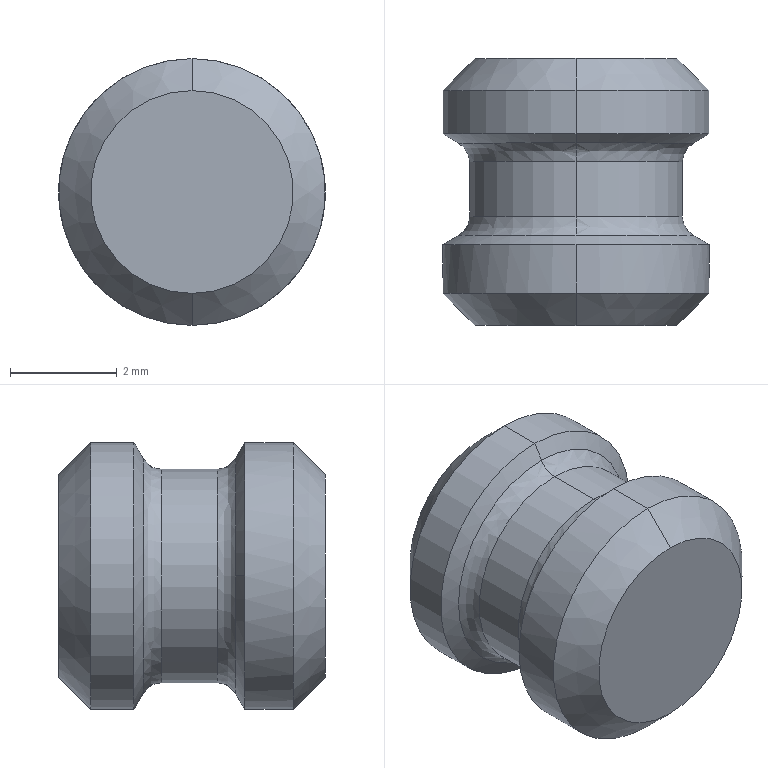Part | SolidWorks | features BaseBody 1 | 1 solid | 44 faces | box 5 x 5 x 5 mm | volume 60.215 mm3 | plane 20 | cone 12 | cylinder 8 | spline 4 | commonest cylinder face diameters 5 x4 2.57 x2 4 x2
STEP:
#1=CARTESIAN_POINT('',(0.,-1.585,2.2));
#2=VERTEX_POINT('',#1);
#3=CARTESIAN_POINT('',(0.,-1.585,-2.2));
#4=VERTEX_POINT('',#3);
#5=CARTESIAN_POINT('',(0.,-1.585,0.));
#6=DIRECTION('',(0.,1.,0.));
#7=DIRECTION('',(0.,0.,1.));
#8=AXIS2_PLACEMENT_3D('',#5,#6,#7);
#9=CIRCLE('',#8,2.2);
#10=EDGE_CURVE('',#2,#4,#9,.T.);
#11=ORIENTED_EDGE('',*,*,#10,.F.);
#12=CARTESIAN_POINT('',(0.,-1.931,2.));
#13=VERTEX_POINT('',#12);
#14=CARTESIAN_POINT('',(0.,-1.931,2.4));
#15=DIRECTION('',(-1.,0.,0.));
#16=DIRECTION('',(0.,0.,1.));
#17=AXIS2_PLACEMENT_3D('',#14,#15,#16);
#18=CIRCLE('',#17,0.4);
#19=EDGE_CURVE('',#2,#13,#18,.T.);
#20=ORIENTED_EDGE('',*,*,#19,.T.);
#21=CARTESIAN_POINT('',(0.,-1.931,-2.));
#22=VERTEX_POINT('',#21);
#23=CARTESIAN_POINT('',(0.,-1.931,0.));
#24=DIRECTION('',(0.,-1.,0.));
#25=DIRECTION('',(0.,0.,-1.));
#26=AXIS2_PLACEMENT_3D('',#23,#24,#25);
#27=CIRCLE('',#26,2.);
#28=EDGE_CURVE('',#22,#13,#27,.T.);
#29=ORIENTED_EDGE('',*,*,#28,.F.);
#30=CARTESIAN_POINT('',(0.,-1.931,-2.4));
#31=DIRECTION('',(1.,0.,0.));
#32=DIRECTION('',(0.,0.,-1.));
#33=AXIS2_PLACEMENT_3D('',#30,#31,#32);
#34=CIRCLE('',#33,0.4);
#35=EDGE_CURVE('',#4,#22,#34,.T.);
#36=ORIENTED_EDGE('',*,*,#35,.F.);
#37=EDGE_LOOP('',(#11,#20,#29,#36));
#38=FACE_OUTER_BOUND('',#37,.T.);
#39=CARTESIAN_POINT('',(0.,-1.585,-2.2));
#40=CARTESIAN_POINT('',(4.4,-1.585,-2.2));
#41=CARTESIAN_POINT('',(4.4,-1.585,2.2));
#42=CARTESIAN_POINT('',(0.,-1.585,2.2));
#43=CARTESIAN_POINT('',(0.,-1.658,-2.073));
#44=CARTESIAN_POINT('',(4.146,-1.658,-2.073));
#45=CARTESIAN_POINT('',(4.146,-1.658,2.073));
#46=CARTESIAN_POINT('',(0.,-1.658,2.073));
#47=CARTESIAN_POINT('',(0.,-1.785,-2.));
#48=CARTESIAN_POINT('',(4.,-1.785,-2.));
#49=CARTESIAN_POINT('',(4.,-1.785,2.));
#50=CARTESIAN_POINT('',(0.,-1.785,2.));
#51=CARTESIAN_POINT('',(0.,-1.931,-2.));
#52=CARTESIAN_POINT('',(4.,-1.931,-2.));
#53=CARTESIAN_POINT('',(4.,-1.931,2.));
#54=CARTESIAN_POINT('',(0.,-1.931,2.));
#55=(BOUNDED_SURFACE()B_SPLINE_SURFACE(3,3,((#39,#40,#41,#42),(#43,#44,#45,#46),(#47,#48,#49,#50),(#51,#52,#53,#54)),.UNSPECIFIED.,.F.,.F.,.T.)B_SPLINE_SURFACE_WITH_KNOTS((4,4),(4,4),(0.,1.),(0.,1.),.UNSPECIFIED.)GEOMETRIC_REPRESENTATION_ITEM()RATIONAL_B_SPLINE_SURFACE(((1.,0.3333,0.3333,1.),(0.9107,0.3036,0.3036,0.9107),(0.9107,0.3036,0.3036,0.9107),(1.,0.3333,0.3333,1.)))REPRESENTATION_ITEM('')SURFACE());
#56=ADVANCED_FACE('',(#38),#55,.F.);
#57=CARTESIAN_POINT('',(0.,-2.969,2.));
#58=VERTEX_POINT('',#57);
#59=CARTESIAN_POINT('',(0.,-2.969,-2.));
#60=VERTEX_POINT('',#59);
#61=CARTESIAN_POINT('',(0.,-2.969,0.));
#62=DIRECTION('',(0.,1.,0.));
#63=DIRECTION('',(0.,0.,1.));
#64=AXIS2_PLACEMENT_3D('',#61,#62,#63);
#65=CIRCLE('',#64,2.);
#66=EDGE_CURVE('',#58,#60,#65,.T.);
#67=ORIENTED_EDGE('',*,*,#66,.F.);
#68=CARTESIAN_POINT('',(0.,-3.315,2.2));
#69=VERTEX_POINT('',#68);
#70=CARTESIAN_POINT('',(0.,-2.969,2.4));
#71=DIRECTION('',(-1.,0.,0.));
#72=DIRECTION('',(0.,0.,1.));
#73=AXIS2_PLACEMENT_3D('',#70,#71,#72);
#74=CIRCLE('',#73,0.4);
#75=EDGE_CURVE('',#58,#69,#74,.T.);
#76=ORIENTED_EDGE('',*,*,#75,.T.);
#77=CARTESIAN_POINT('',(2.2,-3.315,0.));
#78=VERTEX_POINT('',#77);
#79=CARTESIAN_POINT('',(0.,-3.315,0.));
#80=DIRECTION('',(0.,-1.,0.));
#81=DIRECTION('',(0.,0.,-1.));
#82=AXIS2_PLACEMENT_3D('',#79,#80,#81);
#83=CIRCLE('',#82,2.2);
#84=EDGE_CURVE('',#78,#69,#83,.T.);
#85=ORIENTED_EDGE('',*,*,#84,.F.);
#86=CARTESIAN_POINT('',(0.,-3.315,-2.2));
#87=VERTEX_POINT('',#86);
#88=CARTESIAN_POINT('',(0.,-3.315,0.));
#89=DIRECTION('',(0.,-1.,0.));
#90=DIRECTION('',(0.,0.,-1.));
#91=AXIS2_PLACEMENT_3D('',#88,#89,#90);
#92=CIRCLE('',#91,2.2);
#93=EDGE_CURVE('',#87,#78,#92,.T.);
#94=ORIENTED_EDGE('',*,*,#93,.F.);
#95=CARTESIAN_POINT('',(0.,-2.969,-2.4));
#96=DIRECTION('',(1.,0.,0.));
#97=DIRECTION('',(0.,0.,-1.));
#98=AXIS2_PLACEMENT_3D('',#95,#96,#97);
#99=CIRCLE('',#98,0.4);
#100=EDGE_CURVE('',#60,#87,#99,.T.);
#101=ORIENTED_EDGE('',*,*,#100,.F.);
#102=EDGE_LOOP('',(#67,#76,#85,#94,#101));
#103=FACE_OUTER_BOUND('',#102,.T.);
#104=CARTESIAN_POINT('',(0.,-2.969,-2.));
#105=CARTESIAN_POINT('',(4.,-2.969,-2.));
#106=CARTESIAN_POINT('',(4.,-2.969,2.));
#107=CARTESIAN_POINT('',(0.,-2.969,2.));
#108=CARTESIAN_POINT('',(0.,-3.115,-2.));
#109=CARTESIAN_POINT('',(4.,-3.115,-2.));
#110=CARTESIAN_POINT('',(4.,-3.115,2.));
#111=CARTESIAN_POINT('',(0.,-3.115,2.));
#112=CARTESIAN_POINT('',(0.,-3.242,-2.073));
#113=CARTESIAN_POINT('',(4.146,-3.242,-2.073));
#114=CARTESIAN_POINT('',(4.146,-3.242,2.073));
#115=CARTESIAN_POINT('',(0.,-3.242,2.073));
#116=CARTESIAN_POINT('',(0.,-3.315,-2.2));
#117=CARTESIAN_POINT('',(4.4,-3.315,-2.2));
#118=CARTESIAN_POINT('',(4.4,-3.315,2.2));
#119=CARTESIAN_POINT('',(0.,-3.315,2.2));
#120=(BOUNDED_SURFACE()B_SPLINE_SURFACE(3,3,((#104,#105,#106,#107),(#108,#109,#110,#111),(#112,#113,#114,#115),(#116,#117,#118,#119)),.UNSPECIFIED.,.F.,.F.,.T.)B_SPLINE_SURFACE_WITH_KNOTS((4,4),(4,4),(0.,1.),(0.,1.),.UNSPECIFIED.)GEOMETRIC_REPRESENTATION_ITEM()RATIONAL_B_SPLINE_SURFACE(((1.,0.3333,0.3333,1.),(0.9107,0.3036,0.3036,0.9107),(0.9107,0.3036,0.3036,0.9107),(1.,0.3333,0.3333,1.)))REPRESENTATION_ITEM('')SURFACE());
#121=ADVANCED_FACE('',(#103),#120,.F.);
#122=CARTESIAN_POINT('',(0.,-3.458,-1.285));
#123=VERTEX_POINT('',#122);
#124=CARTESIAN_POINT('',(0.,-3.458,1.285));
#125=VERTEX_POINT('',#124);
#126=CARTESIAN_POINT('',(0.,-3.458,0.));
#127=DIRECTION('',(0.,1.,0.));
#128=DIRECTION('',(0.,0.,1.));
#129=AXIS2_PLACEMENT_3D('',#126,#127,#128);
#130=CIRCLE('',#129,1.285);
#131=EDGE_CURVE('',#123,#125,#130,.T.);
#132=ORIENTED_EDGE('',*,*,#131,.F.);
#133=CARTESIAN_POINT('',(0.,-2.5,-1.285));
#134=VERTEX_POINT('',#133);
#135=CARTESIAN_POINT('',(0.,-4.2,-1.285));
#136=DIRECTION('',(0.,1.,0.));
#137=VECTOR('',#136,1000.);
#138=LINE('',#135,#137);
#139=EDGE_CURVE('',#123,#134,#138,.T.);
#140=ORIENTED_EDGE('',*,*,#139,.T.);
#141=CARTESIAN_POINT('',(-0.4116,-2.5,-1.217));
#142=VERTEX_POINT('',#141);
#143=CARTESIAN_POINT('',(0.,-2.5,0.));
#144=DIRECTION('',(0.,-1.,0.));
#145=DIRECTION('',(0.,0.,1.));
#146=AXIS2_PLACEMENT_3D('',#143,#144,#145);
#147=CIRCLE('',#146,1.285);
#148=EDGE_CURVE('',#142,#134,#147,.T.);
#149=ORIENTED_EDGE('',*,*,#148,.F.);
#150=CARTESIAN_POINT('',(-0.4116,-0.153,-1.217));
#151=VERTEX_POINT('',#150);
#152=CARTESIAN_POINT('',(-0.4116,-4.2,-1.217));
#153=DIRECTION('',(0.,-1.,0.));
#154=VECTOR('',#153,1000.);
#155=LINE('',#152,#154);
#156=EDGE_CURVE('',#151,#142,#155,.T.);
#157=ORIENTED_EDGE('',*,*,#156,.F.);
#158=CARTESIAN_POINT('',(-0.8484,-0.153,-0.9651));
#159=VERTEX_POINT('',#158);
#160=CARTESIAN_POINT('',(0.,-0.153,0.));
#161=DIRECTION('',(0.,-1.,0.));
#162=DIRECTION('',(0.,0.,1.));
#163=AXIS2_PLACEMENT_3D('',#160,#161,#162);
#164=CIRCLE('',#163,1.285);
#165=EDGE_CURVE('',#159,#151,#164,.T.);
#166=ORIENTED_EDGE('',*,*,#165,.F.);
#167=CARTESIAN_POINT('',(-0.8484,-2.5,-0.9651));
#168=VERTEX_POINT('',#167);
#169=CARTESIAN_POINT('',(-0.8484,-4.2,-0.9651));
#170=DIRECTION('',(0.,1.,0.));
#171=VECTOR('',#170,1000.);
#172=LINE('',#169,#171);
#173=EDGE_CURVE('',#168,#159,#172,.T.);
#174=ORIENTED_EDGE('',*,*,#173,.F.);
#175=CARTESIAN_POINT('',(-1.26,-2.5,-0.2522));
#176=VERTEX_POINT('',#175);
#177=CARTESIAN_POINT('',(0.,-2.5,0.));
#178=DIRECTION('',(0.,-1.,0.));
#179=DIRECTION('',(0.,0.,1.));
#180=AXIS2_PLACEMENT_3D('',#177,#178,#179);
#181=CIRCLE('',#180,1.285);
#182=EDGE_CURVE('',#176,#168,#181,.T.);
#183=ORIENTED_EDGE('',*,*,#182,.F.);
#184=CARTESIAN_POINT('',(-1.26,-0.153,-0.2522));
#185=VERTEX_POINT('',#184);
#186=CARTESIAN_POINT('',(-1.26,-4.2,-0.2522));
#187=DIRECTION('',(0.,-1.,0.));
#188=VECTOR('',#187,1000.);
#189=LINE('',#186,#188);
#190=EDGE_CURVE('',#185,#176,#189,.T.);
#191=ORIENTED_EDGE('',*,*,#190,.F.);
#192=CARTESIAN_POINT('',(-1.26,-0.153,0.2522));
#193=VERTEX_POINT('',#192);
#194=CARTESIAN_POINT('',(0.,-0.153,0.));
#195=DIRECTION('',(0.,-1.,0.));
#196=DIRECTION('',(0.,0.,1.));
#197=AXIS2_PLACEMENT_3D('',#194,#195,#196);
#198=CIRCLE('',#197,1.285);
#199=EDGE_CURVE('',#193,#185,#198,.T.);
#200=ORIENTED_EDGE('',*,*,#199,.F.);
#201=CARTESIAN_POINT('',(-1.26,-2.5,0.2522));
#202=VERTEX_POINT('',#201);
#203=CARTESIAN_POINT('',(-1.26,-4.2,0.2522));
#204=DIRECTION('',(0.,1.,0.));
#205=VECTOR('',#204,1000.);
#206=LINE('',#203,#205);
#207=EDGE_CURVE('',#202,#193,#206,.T.);
#208=ORIENTED_EDGE('',*,*,#207,.F.);
#209=CARTESIAN_POINT('',(-0.8484,-2.5,0.9651));
#210=VERTEX_POINT('',#209);
#211=CARTESIAN_POINT('',(0.,-2.5,0.));
#212=DIRECTION('',(0.,-1.,0.));
#213=DIRECTION('',(0.,0.,1.));
#214=AXIS2_PLACEMENT_3D('',#211,#212,#213);
#215=CIRCLE('',#214,1.285);
#216=EDGE_CURVE('',#210,#202,#215,.T.);
#217=ORIENTED_EDGE('',*,*,#216,.F.);
#218=CARTESIAN_POINT('',(-0.8484,-0.153,0.9651));
#219=VERTEX_POINT('',#218);
#220=CARTESIAN_POINT('',(-0.8484,-4.2,0.9651));
#221=DIRECTION('',(0.,-1.,0.));
#222=VECTOR('',#221,1000.);
#223=LINE('',#220,#222);
#224=EDGE_CURVE('',#219,#210,#223,.T.);
#225=ORIENTED_EDGE('',*,*,#224,.F.);
#226=CARTESIAN_POINT('',(-0.4116,-0.153,1.217));
#227=VERTEX_POINT('',#226);
#228=CARTESIAN_POINT('',(0.,-0.153,0.));
#229=DIRECTION('',(0.,-1.,0.));
#230=DIRECTION('',(0.,0.,1.));
#231=AXIS2_PLACEMENT_3D('',#228,#229,#230);
#232=CIRCLE('',#231,1.285);
#233=EDGE_CURVE('',#227,#219,#232,.T.);
#234=ORIENTED_EDGE('',*,*,#233,.F.);
#235=CARTESIAN_POINT('',(-0.4116,-2.5,1.217));
#236=VERTEX_POINT('',#235);
#237=CARTESIAN_POINT('',(-0.4116,-4.2,1.217));
#238=DIRECTION('',(0.,1.,0.));
#239=VECTOR('',#238,1000.);
#240=LINE('',#237,#239);
#241=EDGE_CURVE('',#236,#227,#240,.T.);
#242=ORIENTED_EDGE('',*,*,#241,.F.);
#243=CARTESIAN_POINT('',(0.,-2.5,1.285));
#244=VERTEX_POINT('',#243);
#245=CARTESIAN_POINT('',(0.,-2.5,0.));
#246=DIRECTION('',(0.,-1.,0.));
#247=DIRECTION('',(0.,0.,1.));
#248=AXIS2_PLACEMENT_3D('',#245,#246,#247);
#249=CIRCLE('',#248,1.285);
#250=EDGE_CURVE('',#244,#236,#249,.T.);
#251=ORIENTED_EDGE('',*,*,#250,.F.);
#252=CARTESIAN_POINT('',(0.,-4.2,1.285));
#253=DIRECTION('',(0.,1.,0.));
#254=VECTOR('',#253,1000.);
#255=LINE('',#252,#254);
#256=EDGE_CURVE('',#125,#244,#255,.T.);
#257=ORIENTED_EDGE('',*,*,#256,.F.);
#258=EDGE_LOOP('',(#132,#140,#149,#157,#166,#174,#183,#191,#200,#208,#217,#225,#234,#242,#251,#257));
#259=FACE_OUTER_BOUND('',#258,.T.);
#260=CARTESIAN_POINT('',(0.,-4.2,0.));
#261=DIRECTION('',(0.,1.,0.));
#262=DIRECTION('',(0.,0.,1.));
#263=AXIS2_PLACEMENT_3D('',#260,#261,#262);
#264=CYLINDRICAL_SURFACE('',#263,1.285);
#265=ADVANCED_FACE('',(#259),#264,.F.);
#266=CARTESIAN_POINT('',(0.000000029,-0.05489,-1.455));
#267=VERTEX_POINT('',#266);
#268=CARTESIAN_POINT('',(0.000000029,-0.05489,-1.455));
#269=CARTESIAN_POINT('',(-0.135,-0.09989,-1.377));
#270=CARTESIAN_POINT('',(-0.2718,-0.1347,-1.298));
#271=CARTESIAN_POINT('',(-0.4116,-0.153,-1.217));
#272=B_SPLINE_CURVE_WITH_KNOTS('',3,(#268,#269,#270,#271),.UNSPECIFIED.,.F.,.F.,(4,4),(0.,0.0004852),.UNSPECIFIED.);
#273=EDGE_CURVE('',#267,#151,#272,.T.);
#274=ORIENTED_EDGE('',*,*,#273,.F.);
#275=CARTESIAN_POINT('',(0.,0.,-1.55));
#276=VERTEX_POINT('',#275);
#277=CARTESIAN_POINT('',(0.,0.,-1.55));
#278=DIRECTION('',(0.,0.5,-0.866));
#279=VECTOR('',#278,1000.);
#280=LINE('',#277,#279);
#281=EDGE_CURVE('',#267,#276,#280,.T.);
#282=ORIENTED_EDGE('',*,*,#281,.T.);
#283=CARTESIAN_POINT('',(0.,0.,1.55));
#284=VERTEX_POINT('',#283);
#285=CARTESIAN_POINT('',(0.,0.,0.));
#286=DIRECTION('',(0.,-1.,0.));
#287=DIRECTION('',(0.,0.,1.));
#288=AXIS2_PLACEMENT_3D('',#285,#286,#287);
#289=CIRCLE('',#288,1.55);
#290=EDGE_CURVE('',#284,#276,#289,.T.);
#291=ORIENTED_EDGE('',*,*,#290,.F.);
#292=CARTESIAN_POINT('',(0.000000007,-0.05489,1.455));
#293=VERTEX_POINT('',#292);
#294=CARTESIAN_POINT('',(0.,0.,1.55));
#295=DIRECTION('',(0.,0.5,0.866));
#296=VECTOR('',#295,1000.);
#297=LINE('',#294,#296);
#298=EDGE_CURVE('',#293,#284,#297,.T.);
#299=ORIENTED_EDGE('',*,*,#298,.F.);
#300=CARTESIAN_POINT('',(-0.4116,-0.153,1.217));
#301=CARTESIAN_POINT('',(-0.2718,-0.1347,1.298));
#302=CARTESIAN_POINT('',(-0.135,-0.09989,1.377));
#303=CARTESIAN_POINT('',(0.000000007,-0.05489,1.455));
#304=B_SPLINE_CURVE_WITH_KNOTS('',3,(#300,#301,#302,#303),.UNSPECIFIED.,.F.,.F.,(4,4),(0.,0.0004852),.UNSPECIFIED.);
#305=EDGE_CURVE('',#227,#293,#304,.T.);
#306=ORIENTED_EDGE('',*,*,#305,.F.);
#307=ORIENTED_EDGE('',*,*,#233,.T.);
#308=CARTESIAN_POINT('',(-1.26,-0.05489,0.7275));
#309=VERTEX_POINT('',#308);
#310=CARTESIAN_POINT('',(-1.26,-0.05489,0.7275));
#311=CARTESIAN_POINT('',(-1.125,-0.09989,0.8054));
#312=CARTESIAN_POINT('',(-0.9882,-0.1347,0.8844));
#313=CARTESIAN_POINT('',(-0.8484,-0.153,0.9651));
#314=B_SPLINE_CURVE_WITH_KNOTS('',3,(#310,#311,#312,#313),.UNSPECIFIED.,.F.,.F.,(4,4),(0.,0.0004852),.UNSPECIFIED.);
#315=EDGE_CURVE('',#309,#219,#314,.T.);
#316=ORIENTED_EDGE('',*,*,#315,.F.);
#317=CARTESIAN_POINT('',(-1.26,-0.153,0.2522));
#318=CARTESIAN_POINT('',(-1.26,-0.1347,0.4136));
#319=CARTESIAN_POINT('',(-1.26,-0.09989,0.5716));
#320=CARTESIAN_POINT('',(-1.26,-0.05489,0.7275));
#321=B_SPLINE_CURVE_WITH_KNOTS('',3,(#317,#318,#319,#320),.UNSPECIFIED.,.F.,.F.,(4,4),(0.,0.0004852),.UNSPECIFIED.);
#322=EDGE_CURVE('',#193,#309,#321,.T.);
#323=ORIENTED_EDGE('',*,*,#322,.F.);
#324=ORIENTED_EDGE('',*,*,#199,.T.);
#325=CARTESIAN_POINT('',(-1.26,-0.05489,-0.7275));
#326=VERTEX_POINT('',#325);
#327=CARTESIAN_POINT('',(-1.26,-0.05489,-0.7275));
#328=CARTESIAN_POINT('',(-1.26,-0.09989,-0.5716));
#329=CARTESIAN_POINT('',(-1.26,-0.1347,-0.4136));
#330=CARTESIAN_POINT('',(-1.26,-0.153,-0.2522));
#331=B_SPLINE_CURVE_WITH_KNOTS('',3,(#327,#328,#329,#330),.UNSPECIFIED.,.F.,.F.,(4,4),(0.,0.0004852),.UNSPECIFIED.);
#332=EDGE_CURVE('',#326,#185,#331,.T.);
#333=ORIENTED_EDGE('',*,*,#332,.F.);
#334=CARTESIAN_POINT('',(-0.8484,-0.153,-0.9651));
#335=CARTESIAN_POINT('',(-0.9882,-0.1347,-0.8844));
#336=CARTESIAN_POINT('',(-1.125,-0.09989,-0.8054));
#337=CARTESIAN_POINT('',(-1.26,-0.05489,-0.7275));
#338=B_SPLINE_CURVE_WITH_KNOTS('',3,(#334,#335,#336,#337),.UNSPECIFIED.,.F.,.F.,(4,4),(0.,0.0004852),.UNSPECIFIED.);
#339=EDGE_CURVE('',#159,#326,#338,.T.);
#340=ORIENTED_EDGE('',*,*,#339,.F.);
#341=ORIENTED_EDGE('',*,*,#165,.T.);
#342=EDGE_LOOP('',(#274,#282,#291,#299,#306,#307,#316,#323,#324,#333,#340,#341));
#343=FACE_OUTER_BOUND('',#342,.T.);
#344=CARTESIAN_POINT('',(0.,0.,0.));
#345=DIRECTION('',(0.,1.,0.));
#346=DIRECTION('',(0.,0.,1.));
#347=AXIS2_PLACEMENT_3D('',#344,#345,#346);
#348=CONICAL_SURFACE('',#347,1.55,1.047);
#349=ADVANCED_FACE('',(#343),#348,.F.);
#350=CARTESIAN_POINT('',(0.,-4.2,0.));
#351=VERTEX_POINT('',#350);
#352=CARTESIAN_POINT('',(0.,-3.458,1.285));
#353=DIRECTION('',(0.,0.5,0.866));
#354=VECTOR('',#353,1000.);
#355=LINE('',#352,#354);
#356=EDGE_CURVE('',#351,#125,#355,.T.);
#357=ORIENTED_EDGE('',*,*,#356,.F.);
#358=CARTESIAN_POINT('',(0.,-3.458,-1.285));
#359=DIRECTION('',(0.,0.5,-0.866));
#360=VECTOR('',#359,1000.);
#361=LINE('',#358,#360);
#362=EDGE_CURVE('',#351,#123,#361,.T.);
#363=ORIENTED_EDGE('',*,*,#362,.T.);
#364=ORIENTED_EDGE('',*,*,#131,.T.);
#365=EDGE_LOOP('',(#357,#363,#364));
#366=FACE_OUTER_BOUND('',#365,.T.);
#367=CARTESIAN_POINT('',(0.,-3.458,0.));
#368=DIRECTION('',(0.,1.,0.));
#369=DIRECTION('',(0.,0.,1.));
#370=AXIS2_PLACEMENT_3D('',#367,#368,#369);
#371=CONICAL_SURFACE('',#370,1.285,1.047);
#372=ADVANCED_FACE('',(#366),#371,.F.);
#373=CARTESIAN_POINT('',(0.,0.,-1.9));
#374=VERTEX_POINT('',#373);
#375=CARTESIAN_POINT('',(0.,0.,1.9));
#376=VERTEX_POINT('',#375);
#377=CARTESIAN_POINT('',(0.,0.,0.));
#378=DIRECTION('',(0.,-1.,0.));
#379=DIRECTION('',(0.,0.,-1.));
#380=AXIS2_PLACEMENT_3D('',#377,#378,#379);
#381=CIRCLE('',#380,1.9);
#382=EDGE_CURVE('',#374,#376,#381,.T.);
#383=ORIENTED_EDGE('',*,*,#382,.T.);
#384=CARTESIAN_POINT('',(0.,-0.6,2.5));
#385=VERTEX_POINT('',#384);
#386=CARTESIAN_POINT('',(0.,-0.6,2.5));
#387=DIRECTION('',(0.,-0.7071,0.7071));
#388=VECTOR('',#387,1000.);
#389=LINE('',#386,#388);
#390=EDGE_CURVE('',#376,#385,#389,.T.);
#391=ORIENTED_EDGE('',*,*,#390,.T.);
#392=CARTESIAN_POINT('',(0.,-0.6,-2.5));
#393=VERTEX_POINT('',#392);
#394=CARTESIAN_POINT('',(0.,-0.6,0.));
#395=DIRECTION('',(0.,1.,0.));
#396=DIRECTION('',(0.,0.,-1.));
#397=AXIS2_PLACEMENT_3D('',#394,#395,#396);
#398=CIRCLE('',#397,2.5);
#399=EDGE_CURVE('',#385,#393,#398,.T.);
#400=ORIENTED_EDGE('',*,*,#399,.T.);
#401=CARTESIAN_POINT('',(0.,-0.6,-2.5));
#402=DIRECTION('',(0.,-0.7071,-0.7071));
#403=VECTOR('',#402,1000.);
#404=LINE('',#401,#403);
#405=EDGE_CURVE('',#374,#393,#404,.T.);
#406=ORIENTED_EDGE('',*,*,#405,.F.);
#407=EDGE_LOOP('',(#383,#391,#400,#406));
#408=FACE_OUTER_BOUND('',#407,.T.);
#409=CARTESIAN_POINT('',(0.,-0.6,0.));
#410=DIRECTION('',(0.,-1.,0.));
#411=DIRECTION('',(0.,0.,-1.));
#412=AXIS2_PLACEMENT_3D('',#409,#410,#411);
#413=CONICAL_SURFACE('',#412,2.5,0.7854);
#414=ADVANCED_FACE('',(#408),#413,.T.);
#415=CARTESIAN_POINT('',(0.,-1.411,2.5));
#416=VERTEX_POINT('',#415);
#417=CARTESIAN_POINT('',(0.,-1.411,-2.5));
#418=VERTEX_POINT('',#417);
#419=CARTESIAN_POINT('',(0.,-1.411,0.));
#420=DIRECTION('',(0.,1.,0.));
#421=DIRECTION('',(0.,0.,1.));
#422=AXIS2_PLACEMENT_3D('',#419,#420,#421);
#423=CIRCLE('',#422,2.5);
#424=EDGE_CURVE('',#416,#418,#423,.T.);
#425=ORIENTED_EDGE('',*,*,#424,.T.);
#426=CARTESIAN_POINT('',(0.,-5.,-2.5));
#427=DIRECTION('',(0.,1.,0.));
#428=VECTOR('',#427,1000.);
#429=LINE('',#426,#428);
#430=EDGE_CURVE('',#418,#393,#429,.T.);
#431=ORIENTED_EDGE('',*,*,#430,.T.);
#432=ORIENTED_EDGE('',*,*,#399,.F.);
#433=CARTESIAN_POINT('',(0.,-5.,2.5));
#434=DIRECTION('',(0.,1.,0.));
#435=VECTOR('',#434,1000.);
#436=LINE('',#433,#435);
#437=EDGE_CURVE('',#416,#385,#436,.T.);
#438=ORIENTED_EDGE('',*,*,#437,.F.);
#439=EDGE_LOOP('',(#425,#431,#432,#438));
#440=FACE_OUTER_BOUND('',#439,.T.);
#441=CARTESIAN_POINT('',(0.,-5.,0.));
#442=DIRECTION('',(0.,1.,0.));
#443=DIRECTION('',(0.,0.,1.));
#444=AXIS2_PLACEMENT_3D('',#441,#442,#443);
#445=CYLINDRICAL_SURFACE('',#444,2.5);
#446=ADVANCED_FACE('',(#440),#445,.T.);
#447=ORIENTED_EDGE('',*,*,#10,.T.);
#448=CARTESIAN_POINT('',(0.,-1.411,-2.5));
#449=DIRECTION('',(0.,0.5,-0.866));
#450=VECTOR('',#449,1000.);
#451=LINE('',#448,#450);
#452=EDGE_CURVE('',#4,#418,#451,.T.);
#453=ORIENTED_EDGE('',*,*,#452,.T.);
#454=ORIENTED_EDGE('',*,*,#424,.F.);
#455=CARTESIAN_POINT('',(0.,-1.411,2.5));
#456=DIRECTION('',(0.,0.5,0.866));
#457=VECTOR('',#456,1000.);
#458=LINE('',#455,#457);
#459=EDGE_CURVE('',#2,#416,#458,.T.);
#460=ORIENTED_EDGE('',*,*,#459,.F.);
#461=EDGE_LOOP('',(#447,#453,#454,#460));
#462=FACE_OUTER_BOUND('',#461,.T.);
#463=CARTESIAN_POINT('',(0.,-1.411,0.));
#464=DIRECTION('',(0.,1.,0.));
#465=DIRECTION('',(0.,0.,1.));
#466=AXIS2_PLACEMENT_3D('',#463,#464,#465);
#467=CONICAL_SURFACE('',#466,2.5,1.047);
#468=ADVANCED_FACE('',(#462),#467,.T.);
#469=ORIENTED_EDGE('',*,*,#66,.T.);
#470=CARTESIAN_POINT('',(0.,-5.,-2.));
#471=DIRECTION('',(0.,1.,0.));
#472=VECTOR('',#471,1000.);
#473=LINE('',#470,#472);
#474=EDGE_CURVE('',#60,#22,#473,.T.);
#475=ORIENTED_EDGE('',*,*,#474,.T.);
#476=ORIENTED_EDGE('',*,*,#28,.T.);
#477=CARTESIAN_POINT('',(0.,-5.,2.));
#478=DIRECTION('',(0.,1.,0.));
#479=VECTOR('',#478,1000.);
#480=LINE('',#477,#479);
#481=EDGE_CURVE('',#58,#13,#480,.T.);
#482=ORIENTED_EDGE('',*,*,#481,.F.);
#483=EDGE_LOOP('',(#469,#475,#476,#482));
#484=FACE_OUTER_BOUND('',#483,.T.);
#485=CARTESIAN_POINT('',(0.,-5.,0.));
#486=DIRECTION('',(0.,1.,0.));
#487=DIRECTION('',(0.,0.,1.));
#488=AXIS2_PLACEMENT_3D('',#485,#486,#487);
#489=CYLINDRICAL_SURFACE('',#488,2.);
#490=ADVANCED_FACE('',(#484),#489,.T.);
#491=ORIENTED_EDGE('',*,*,#84,.T.);
#492=CARTESIAN_POINT('',(-2.2,-3.315,0.));
#493=VERTEX_POINT('',#492);
#494=CARTESIAN_POINT('',(0.,-3.315,0.));
#495=DIRECTION('',(0.,-1.,0.));
#496=DIRECTION('',(0.,0.,-1.));
#497=AXIS2_PLACEMENT_3D('',#494,#495,#496);
#498=CIRCLE('',#497,2.2);
#499=EDGE_CURVE('',#69,#493,#498,.T.);
#500=ORIENTED_EDGE('',*,*,#499,.T.);
#501=CARTESIAN_POINT('',(-2.5,-3.489,0.));
#502=VERTEX_POINT('',#501);
#503=CARTESIAN_POINT('',(-2.5,-3.489,0.));
#504=DIRECTION('',(-0.866,-0.5,0.));
#505=VECTOR('',#504,1000.);
#506=LINE('',#503,#505);
#507=EDGE_CURVE('',#493,#502,#506,.T.);
#508=ORIENTED_EDGE('',*,*,#507,.T.);
#509=CARTESIAN_POINT('',(0.,-3.489,2.5));
#510=VERTEX_POINT('',#509);
#511=CARTESIAN_POINT('',(0.,-3.489,0.));
#512=DIRECTION('',(0.,1.,0.));
#513=DIRECTION('',(0.,0.,-1.));
#514=AXIS2_PLACEMENT_3D('',#511,#512,#513);
#515=CIRCLE('',#514,2.5);
#516=EDGE_CURVE('',#502,#510,#515,.T.);
#517=ORIENTED_EDGE('',*,*,#516,.T.);
#518=CARTESIAN_POINT('',(2.5,-3.489,0.));
#519=VERTEX_POINT('',#518);
#520=CARTESIAN_POINT('',(0.,-3.489,0.));
#521=DIRECTION('',(0.,1.,0.));
#522=DIRECTION('',(0.,0.,-1.));
#523=AXIS2_PLACEMENT_3D('',#520,#521,#522);
#524=CIRCLE('',#523,2.5);
#525=EDGE_CURVE('',#510,#519,#524,.T.);
#526=ORIENTED_EDGE('',*,*,#525,.T.);
#527=CARTESIAN_POINT('',(2.5,-3.489,0.));
#528=DIRECTION('',(0.866,-0.5,0.));
#529=VECTOR('',#528,1000.);
#530=LINE('',#527,#529);
#531=EDGE_CURVE('',#78,#519,#530,.T.);
#532=ORIENTED_EDGE('',*,*,#531,.F.);
#533=EDGE_LOOP('',(#491,#500,#508,#517,#526,#532));
#534=FACE_OUTER_BOUND('',#533,.T.);
#535=CARTESIAN_POINT('',(0.,-3.489,0.));
#536=DIRECTION('',(0.,-1.,0.));
#537=DIRECTION('',(1.,0.,0.));
#538=AXIS2_PLACEMENT_3D('',#535,#536,#537);
#539=CONICAL_SURFACE('',#538,2.5,1.047);
#540=ADVANCED_FACE('',(#534),#539,.T.);
#541=CARTESIAN_POINT('',(0.,-4.4,2.5));
#542=VERTEX_POINT('',#541);
#543=CARTESIAN_POINT('',(0.,-4.4,-2.5));
#544=VERTEX_POINT('',#543);
#545=CARTESIAN_POINT('',(0.,-4.4,0.));
#546=DIRECTION('',(0.,1.,0.));
#547=DIRECTION('',(0.,0.,1.));
#548=AXIS2_PLACEMENT_3D('',#545,#546,#547);
#549=CIRCLE('',#548,2.5);
#550=EDGE_CURVE('',#542,#544,#549,.T.);
#551=ORIENTED_EDGE('',*,*,#550,.T.);
#552=CARTESIAN_POINT('',(0.,-3.489,-2.5));
#553=VERTEX_POINT('',#552);
#554=CARTESIAN_POINT('',(0.,-5.,-2.5));
#555=DIRECTION('',(0.,1.,0.));
#556=VECTOR('',#555,1000.);
#557=LINE('',#554,#556);
#558=EDGE_CURVE('',#544,#553,#557,.T.);
#559=ORIENTED_EDGE('',*,*,#558,.T.);
#560=CARTESIAN_POINT('',(0.,-3.489,0.));
#561=DIRECTION('',(0.,1.,0.));
#562=DIRECTION('',(0.,0.,-1.));
#563=AXIS2_PLACEMENT_3D('',#560,#561,#562);
#564=CIRCLE('',#563,2.5);
#565=EDGE_CURVE('',#519,#553,#564,.T.);
#566=ORIENTED_EDGE('',*,*,#565,.F.);
#567=ORIENTED_EDGE('',*,*,#525,.F.);
#568=CARTESIAN_POINT('',(0.,-5.,2.5));
#569=DIRECTION('',(0.,1.,0.));
#570=VECTOR('',#569,1000.);
#571=LINE('',#568,#570);
#572=EDGE_CURVE('',#542,#510,#571,.T.);
#573=ORIENTED_EDGE('',*,*,#572,.F.);
#574=EDGE_LOOP('',(#551,#559,#566,#567,#573));
#575=FACE_OUTER_BOUND('',#574,.T.);
#576=CARTESIAN_POINT('',(0.,-5.,0.));
#577=DIRECTION('',(0.,1.,0.));
#578=DIRECTION('',(0.,0.,1.));
#579=AXIS2_PLACEMENT_3D('',#576,#577,#578);
#580=CYLINDRICAL_SURFACE('',#579,2.5);
#581=ADVANCED_FACE('',(#575),#580,.T.);
#582=CARTESIAN_POINT('',(0.,-5.,1.9));
#583=VERTEX_POINT('',#582);
#584=CARTESIAN_POINT('',(0.,-5.,-1.9));
#585=VERTEX_POINT('',#584);
#586=CARTESIAN_POINT('',(0.,-5.,0.));
#587=DIRECTION('',(0.,1.,0.));
#588=DIRECTION('',(0.,0.,1.));
#589=AXIS2_PLACEMENT_3D('',#586,#587,#588);
#590=CIRCLE('',#589,1.9);
#591=EDGE_CURVE('',#583,#585,#590,.T.);
#592=ORIENTED_EDGE('',*,*,#591,.T.);
#593=CARTESIAN_POINT('',(0.,-4.4,-2.5));
#594=DIRECTION('',(0.,0.7071,-0.7071));
#595=VECTOR('',#594,1000.);
#596=LINE('',#593,#595);
#597=EDGE_CURVE('',#585,#544,#596,.T.);
#598=ORIENTED_EDGE('',*,*,#597,.T.);
#599=ORIENTED_EDGE('',*,*,#550,.F.);
#600=CARTESIAN_POINT('',(0.,-4.4,2.5));
#601=DIRECTION('',(0.,0.7071,0.7071));
#602=VECTOR('',#601,1000.);
#603=LINE('',#600,#602);
#604=EDGE_CURVE('',#583,#542,#603,.T.);
#605=ORIENTED_EDGE('',*,*,#604,.F.);
#606=EDGE_LOOP('',(#592,#598,#599,#605));
#607=FACE_OUTER_BOUND('',#606,.T.);
#608=CARTESIAN_POINT('',(0.,-4.4,0.));
#609=DIRECTION('',(0.,1.,0.));
#610=DIRECTION('',(0.,0.,1.));
#611=AXIS2_PLACEMENT_3D('',#608,#609,#610);
#612=CONICAL_SURFACE('',#611,2.5,0.7854);
#613=ADVANCED_FACE('',(#607),#612,.T.);
#614=ORIENTED_EDGE('',*,*,#139,.F.);
#615=CARTESIAN_POINT('',(0.,-3.458,0.));
#616=DIRECTION('',(0.,1.,0.));
#617=DIRECTION('',(0.,0.,1.));
#618=AXIS2_PLACEMENT_3D('',#615,#616,#617);
#619=CIRCLE('',#618,1.285);
#620=EDGE_CURVE('',#125,#123,#619,.T.);
#621=ORIENTED_EDGE('',*,*,#620,.F.);
#622=ORIENTED_EDGE('',*,*,#256,.T.);
#623=CARTESIAN_POINT('',(0.4116,-2.5,1.217));
#624=VERTEX_POINT('',#623);
#625=CARTESIAN_POINT('',(0.,-2.5,0.));
#626=DIRECTION('',(0.,-1.,0.));
#627=DIRECTION('',(0.,0.,1.));
#628=AXIS2_PLACEMENT_3D('',#625,#626,#627);
#629=CIRCLE('',#628,1.285);
#630=EDGE_CURVE('',#624,#244,#629,.T.);
#631=ORIENTED_EDGE('',*,*,#630,.F.);
#632=CARTESIAN_POINT('',(0.4116,-0.153,1.217));
#633=VERTEX_POINT('',#632);
#634=CARTESIAN_POINT('',(0.4116,-4.2,1.217));
#635=DIRECTION('',(0.,-1.,0.));
#636=VECTOR('',#635,1000.);
#637=LINE('',#634,#636);
#638=EDGE_CURVE('',#633,#624,#637,.T.);
#639=ORIENTED_EDGE('',*,*,#638,.F.);
#640=CARTESIAN_POINT('',(0.8484,-0.153,0.9651));
#641=VERTEX_POINT('',#640);
#642=CARTESIAN_POINT('',(0.,-0.153,0.));
#643=DIRECTION('',(0.,-1.,0.));
#644=DIRECTION('',(0.,0.,1.));
#645=AXIS2_PLACEMENT_3D('',#642,#643,#644);
#646=CIRCLE('',#645,1.285);
#647=EDGE_CURVE('',#641,#633,#646,.T.);
#648=ORIENTED_EDGE('',*,*,#647,.F.);
#649=CARTESIAN_POINT('',(0.8484,-2.5,0.9651));
#650=VERTEX_POINT('',#649);
#651=CARTESIAN_POINT('',(0.8484,-4.2,0.9651));
#652=DIRECTION('',(0.,1.,0.));
#653=VECTOR('',#652,1000.);
#654=LINE('',#651,#653);
#655=EDGE_CURVE('',#650,#641,#654,.T.);
#656=ORIENTED_EDGE('',*,*,#655,.F.);
#657=CARTESIAN_POINT('',(1.26,-2.5,0.2522));
#658=VERTEX_POINT('',#657);
#659=CARTESIAN_POINT('',(0.,-2.5,0.));
#660=DIRECTION('',(0.,-1.,0.));
#661=DIRECTION('',(0.,0.,1.));
#662=AXIS2_PLACEMENT_3D('',#659,#660,#661);
#663=CIRCLE('',#662,1.285);
#664=EDGE_CURVE('',#658,#650,#663,.T.);
#665=ORIENTED_EDGE('',*,*,#664,.F.);
#666=CARTESIAN_POINT('',(1.26,-0.153,0.2522));
#667=VERTEX_POINT('',#666);
#668=CARTESIAN_POINT('',(1.26,-4.2,0.2522));
#669=DIRECTION('',(0.,-1.,0.));
#670=VECTOR('',#669,1000.);
#671=LINE('',#668,#670);
#672=EDGE_CURVE('',#667,#658,#671,.T.);
#673=ORIENTED_EDGE('',*,*,#672,.F.);
#674=CARTESIAN_POINT('',(1.26,-0.153,-0.2522));
#675=VERTEX_POINT('',#674);
#676=CARTESIAN_POINT('',(0.,-0.153,0.));
#677=DIRECTION('',(0.,-1.,0.));
#678=DIRECTION('',(0.,0.,1.));
#679=AXIS2_PLACEMENT_3D('',#676,#677,#678);
#680=CIRCLE('',#679,1.285);
#681=EDGE_CURVE('',#675,#667,#680,.T.);
#682=ORIENTED_EDGE('',*,*,#681,.F.);
#683=CARTESIAN_POINT('',(1.26,-2.5,-0.2522));
#684=VERTEX_POINT('',#683);
#685=CARTESIAN_POINT('',(1.26,-4.2,-0.2522));
#686=DIRECTION('',(0.,1.,0.));
#687=VECTOR('',#686,1000.);
#688=LINE('',#685,#687);
#689=EDGE_CURVE('',#684,#675,#688,.T.);
#690=ORIENTED_EDGE('',*,*,#689,.F.);
#691=CARTESIAN_POINT('',(0.8484,-2.5,-0.9651));
#692=VERTEX_POINT('',#691);
#693=CARTESIAN_POINT('',(0.,-2.5,0.));
#694=DIRECTION('',(0.,-1.,0.));
#695=DIRECTION('',(0.,0.,1.));
#696=AXIS2_PLACEMENT_3D('',#693,#694,#695);
#697=CIRCLE('',#696,1.285);
#698=EDGE_CURVE('',#692,#684,#697,.T.);
#699=ORIENTED_EDGE('',*,*,#698,.F.);
#700=CARTESIAN_POINT('',(0.8484,-0.153,-0.9651));
#701=VERTEX_POINT('',#700);
#702=CARTESIAN_POINT('',(0.8484,-4.2,-0.9651));
#703=DIRECTION('',(0.,-1.,0.));
#704=VECTOR('',#703,1000.);
#705=LINE('',#702,#704);
#706=EDGE_CURVE('',#701,#692,#705,.T.);
#707=ORIENTED_EDGE('',*,*,#706,.F.);
#708=CARTESIAN_POINT('',(0.4116,-0.153,-1.217));
#709=VERTEX_POINT('',#708);
#710=CARTESIAN_POINT('',(0.,-0.153,0.));
#711=DIRECTION('',(0.,-1.,0.));
#712=DIRECTION('',(0.,0.,1.));
#713=AXIS2_PLACEMENT_3D('',#710,#711,#712);
#714=CIRCLE('',#713,1.285);
#715=EDGE_CURVE('',#709,#701,#714,.T.);
#716=ORIENTED_EDGE('',*,*,#715,.F.);
#717=CARTESIAN_POINT('',(0.4116,-2.5,-1.217));
#718=VERTEX_POINT('',#717);
#719=CARTESIAN_POINT('',(0.4116,-4.2,-1.217));
#720=DIRECTION('',(0.,1.,0.));
#721=VECTOR('',#720,1000.);
#722=LINE('',#719,#721);
#723=EDGE_CURVE('',#718,#709,#722,.T.);
#724=ORIENTED_EDGE('',*,*,#723,.F.);
#725=CARTESIAN_POINT('',(0.,-2.5,0.));
#726=DIRECTION('',(0.,-1.,0.));
#727=DIRECTION('',(0.,0.,1.));
#728=AXIS2_PLACEMENT_3D('',#725,#726,#727);
#729=CIRCLE('',#728,1.285);
#730=EDGE_CURVE('',#134,#718,#729,.T.);
#731=ORIENTED_EDGE('',*,*,#730,.F.);
#732=EDGE_LOOP('',(#614,#621,#622,#631,#639,#648,#656,#665,#673,#682,#690,#699,#707,#716,#724,#731));
#733=FACE_OUTER_BOUND('',#732,.T.);
#734=CARTESIAN_POINT('',(0.,-4.2,0.));
#735=DIRECTION('',(0.,1.,0.));
#736=DIRECTION('',(0.,0.,1.));
#737=AXIS2_PLACEMENT_3D('',#734,#735,#736);
#738=CYLINDRICAL_SURFACE('',#737,1.285);
#739=ADVANCED_FACE('',(#733),#738,.F.);
#740=CARTESIAN_POINT('',(1.26,-2.5,0.7275));
#741=VERTEX_POINT('',#740);
#742=CARTESIAN_POINT('',(1.26,-0.05489,0.7275));
#743=VERTEX_POINT('',#742);
#744=CARTESIAN_POINT('',(1.26,-2.5,0.7275));
#745=DIRECTION('',(0.,1.,0.));
#746=VECTOR('',#745,1000.);
#747=LINE('',#744,#746);
#748=EDGE_CURVE('',#741,#743,#747,.T.);
#749=ORIENTED_EDGE('',*,*,#748,.F.);
#750=CARTESIAN_POINT('',(0.,-2.5,1.455));
#751=DIRECTION('',(0.866,0.,-0.5));
#752=VECTOR('',#751,1000.);
#753=LINE('',#750,#752);
#754=EDGE_CURVE('',#650,#741,#753,.T.);
#755=ORIENTED_EDGE('',*,*,#754,.F.);
#756=ORIENTED_EDGE('',*,*,#655,.T.);
#757=CARTESIAN_POINT('',(1.26,-0.05489,0.7275));
#758=CARTESIAN_POINT('',(1.125,-0.09989,0.8054));
#759=CARTESIAN_POINT('',(0.9882,-0.1347,0.8844));
#760=CARTESIAN_POINT('',(0.8484,-0.153,0.9651));
#761=B_SPLINE_CURVE_WITH_KNOTS('',3,(#757,#758,#759,#760),.UNSPECIFIED.,.F.,.F.,(4,4),(0.,0.0004852),.UNSPECIFIED.);
#762=EDGE_CURVE('',#743,#641,#761,.T.);
#763=ORIENTED_EDGE('',*,*,#762,.F.);
#764=EDGE_LOOP('',(#749,#755,#756,#763));
#765=FACE_OUTER_BOUND('',#764,.T.);
#766=CARTESIAN_POINT('',(0.,-2.5,1.455));
#767=DIRECTION('',(0.5,0.,0.866));
#768=DIRECTION('',(0.866,0.,-0.5));
#769=AXIS2_PLACEMENT_3D('',#766,#767,#768);
#770=PLANE('',#769);
#771=ADVANCED_FACE('',(#765),#770,.F.);
#772=CARTESIAN_POINT('',(1.26,-2.5,0.));
#773=DIRECTION('',(0.,0.,-1.));
#774=VECTOR('',#773,1000.);
#775=LINE('',#772,#774);
#776=EDGE_CURVE('',#741,#658,#775,.T.);
#777=ORIENTED_EDGE('',*,*,#776,.T.);
#778=ORIENTED_EDGE('',*,*,#664,.T.);
#779=ORIENTED_EDGE('',*,*,#754,.T.);
#780=EDGE_LOOP('',(#777,#778,#779));
#781=FACE_OUTER_BOUND('',#780,.T.);
#782=CARTESIAN_POINT('',(0.,-2.5,0.));
#783=DIRECTION('',(0.,1.,0.));
#784=DIRECTION('',(0.,0.,1.));
#785=AXIS2_PLACEMENT_3D('',#782,#783,#784);
#786=PLANE('',#785);
#787=ADVANCED_FACE('',(#781),#786,.T.);
#788=ORIENTED_EDGE('',*,*,#672,.T.);
#789=ORIENTED_EDGE('',*,*,#776,.F.);
#790=ORIENTED_EDGE('',*,*,#748,.T.);
#791=CARTESIAN_POINT('',(1.26,-0.153,0.2522));
#792=CARTESIAN_POINT('',(1.26,-0.1347,0.4136));
#793=CARTESIAN_POINT('',(1.26,-0.09989,0.5716));
#794=CARTESIAN_POINT('',(1.26,-0.05489,0.7275));
#795=B_SPLINE_CURVE_WITH_KNOTS('',3,(#791,#792,#793,#794),.UNSPECIFIED.,.F.,.F.,(4,4),(0.,0.0004852),.UNSPECIFIED.);
#796=EDGE_CURVE('',#667,#743,#795,.T.);
#797=ORIENTED_EDGE('',*,*,#796,.F.);
#798=EDGE_LOOP('',(#788,#789,#790,#797));
#799=FACE_OUTER_BOUND('',#798,.T.);
#800=CARTESIAN_POINT('',(1.26,-2.5,0.7275));
#801=DIRECTION('',(1.,0.,0.));
#802=DIRECTION('',(0.,0.,-1.));
#803=AXIS2_PLACEMENT_3D('',#800,#801,#802);
#804=PLANE('',#803);
#805=ADVANCED_FACE('',(#799),#804,.F.);
#806=ORIENTED_EDGE('',*,*,#281,.F.);
#807=CARTESIAN_POINT('',(0.4116,-0.153,-1.217));
#808=CARTESIAN_POINT('',(0.2718,-0.1347,-1.298));
#809=CARTESIAN_POINT('',(0.135,-0.09989,-1.377));
#810=CARTESIAN_POINT('',(0.000000029,-0.05489,-1.455));
#811=B_SPLINE_CURVE_WITH_KNOTS('',3,(#807,#808,#809,#810),.UNSPECIFIED.,.F.,.F.,(4,4),(0.,0.0004852),.UNSPECIFIED.);
#812=EDGE_CURVE('',#709,#267,#811,.T.);
#813=ORIENTED_EDGE('',*,*,#812,.F.);
#814=ORIENTED_EDGE('',*,*,#715,.T.);
#815=CARTESIAN_POINT('',(1.26,-0.05489,-0.7275));
#816=VERTEX_POINT('',#815);
#817=CARTESIAN_POINT('',(1.26,-0.05489,-0.7275));
#818=CARTESIAN_POINT('',(1.125,-0.09989,-0.8054));
#819=CARTESIAN_POINT('',(0.9882,-0.1347,-0.8844));
#820=CARTESIAN_POINT('',(0.8484,-0.153,-0.9651));
#821=B_SPLINE_CURVE_WITH_KNOTS('',3,(#817,#818,#819,#820),.UNSPECIFIED.,.F.,.F.,(4,4),(0.,0.0004852),.UNSPECIFIED.);
#822=EDGE_CURVE('',#816,#701,#821,.T.);
#823=ORIENTED_EDGE('',*,*,#822,.F.);
#824=CARTESIAN_POINT('',(1.26,-0.153,-0.2522));
#825=CARTESIAN_POINT('',(1.26,-0.1347,-0.4136));
#826=CARTESIAN_POINT('',(1.26,-0.09989,-0.5716));
#827=CARTESIAN_POINT('',(1.26,-0.05489,-0.7275));
#828=B_SPLINE_CURVE_WITH_KNOTS('',3,(#824,#825,#826,#827),.UNSPECIFIED.,.F.,.F.,(4,4),(0.,0.0004852),.UNSPECIFIED.);
#829=EDGE_CURVE('',#675,#816,#828,.T.);
#830=ORIENTED_EDGE('',*,*,#829,.F.);
#831=ORIENTED_EDGE('',*,*,#681,.T.);
#832=ORIENTED_EDGE('',*,*,#796,.T.);
#833=ORIENTED_EDGE('',*,*,#762,.T.);
#834=ORIENTED_EDGE('',*,*,#647,.T.);
#835=CARTESIAN_POINT('',(0.000000007,-0.05489,1.455));
#836=CARTESIAN_POINT('',(0.135,-0.09989,1.377));
#837=CARTESIAN_POINT('',(0.2718,-0.1347,1.298));
#838=CARTESIAN_POINT('',(0.4116,-0.153,1.217));
#839=B_SPLINE_CURVE_WITH_KNOTS('',3,(#835,#836,#837,#838),.UNSPECIFIED.,.F.,.F.,(4,4),(0.,0.0004852),.UNSPECIFIED.);
#840=EDGE_CURVE('',#293,#633,#839,.T.);
#841=ORIENTED_EDGE('',*,*,#840,.F.);
#842=ORIENTED_EDGE('',*,*,#298,.T.);
#843=CARTESIAN_POINT('',(0.,0.,0.));
#844=DIRECTION('',(0.,-1.,0.));
#845=DIRECTION('',(0.,0.,1.));
#846=AXIS2_PLACEMENT_3D('',#843,#844,#845);
#847=CIRCLE('',#846,1.55);
#848=EDGE_CURVE('',#276,#284,#847,.T.);
#849=ORIENTED_EDGE('',*,*,#848,.F.);
#850=EDGE_LOOP('',(#806,#813,#814,#823,#830,#831,#832,#833,#834,#841,#842,#849));
#851=FACE_OUTER_BOUND('',#850,.T.);
#852=CARTESIAN_POINT('',(0.,0.,0.));
#853=DIRECTION('',(0.,1.,0.));
#854=DIRECTION('',(0.,0.,1.));
#855=AXIS2_PLACEMENT_3D('',#852,#853,#854);
#856=CONICAL_SURFACE('',#855,1.55,1.047);
#857=ADVANCED_FACE('',(#851),#856,.F.);
#858=CARTESIAN_POINT('',(1.26,-2.5,-0.7275));
#859=VERTEX_POINT('',#858);
#860=CARTESIAN_POINT('',(1.26,-2.5,-0.7275));
#861=DIRECTION('',(0.,1.,0.));
#862=VECTOR('',#861,1000.);
#863=LINE('',#860,#862);
#864=EDGE_CURVE('',#859,#816,#863,.T.);
#865=ORIENTED_EDGE('',*,*,#864,.F.);
#866=CARTESIAN_POINT('',(1.26,-2.5,0.7275));
#867=DIRECTION('',(0.,0.,-1.));
#868=VECTOR('',#867,1000.);
#869=LINE('',#866,#868);
#870=EDGE_CURVE('',#684,#859,#869,.T.);
#871=ORIENTED_EDGE('',*,*,#870,.F.);
#872=ORIENTED_EDGE('',*,*,#689,.T.);
#873=ORIENTED_EDGE('',*,*,#829,.T.);
#874=EDGE_LOOP('',(#865,#871,#872,#873));
#875=FACE_OUTER_BOUND('',#874,.T.);
#876=CARTESIAN_POINT('',(1.26,-2.5,0.7275));
#877=DIRECTION('',(1.,0.,0.));
#878=DIRECTION('',(0.,0.,-1.));
#879=AXIS2_PLACEMENT_3D('',#876,#877,#878);
#880=PLANE('',#879);
#881=ADVANCED_FACE('',(#875),#880,.F.);
#882=CARTESIAN_POINT('',(1.26,-2.5,-0.7275));
#883=DIRECTION('',(-0.866,0.,-0.5));
#884=VECTOR('',#883,1000.);
#885=LINE('',#882,#884);
#886=EDGE_CURVE('',#859,#692,#885,.T.);
#887=ORIENTED_EDGE('',*,*,#886,.T.);
#888=ORIENTED_EDGE('',*,*,#698,.T.);
#889=ORIENTED_EDGE('',*,*,#870,.T.);
#890=EDGE_LOOP('',(#887,#888,#889));
#891=FACE_OUTER_BOUND('',#890,.T.);
#892=CARTESIAN_POINT('',(0.,-2.5,0.));
#893=DIRECTION('',(0.,1.,0.));
#894=DIRECTION('',(0.,0.,1.));
#895=AXIS2_PLACEMENT_3D('',#892,#893,#894);
#896=PLANE('',#895);
#897=ADVANCED_FACE('',(#891),#896,.T.);
#898=ORIENTED_EDGE('',*,*,#706,.T.);
#899=ORIENTED_EDGE('',*,*,#886,.F.);
#900=ORIENTED_EDGE('',*,*,#864,.T.);
#901=ORIENTED_EDGE('',*,*,#822,.T.);
#902=EDGE_LOOP('',(#898,#899,#900,#901));
#903=FACE_OUTER_BOUND('',#902,.T.);
#904=CARTESIAN_POINT('',(1.26,-2.5,-0.7275));
#905=DIRECTION('',(0.5,0.,-0.866));
#906=DIRECTION('',(-0.866,0.,-0.5));
#907=AXIS2_PLACEMENT_3D('',#904,#905,#906);
#908=PLANE('',#907);
#909=ADVANCED_FACE('',(#903),#908,.F.);
#910=CARTESIAN_POINT('',(0.,-2.5,-1.455));
#911=VERTEX_POINT('',#910);
#912=CARTESIAN_POINT('',(0.,-2.5,-1.455));
#913=DIRECTION('',(0.,1.,0.));
#914=VECTOR('',#913,1000.);
#915=LINE('',#912,#914);
#916=EDGE_CURVE('',#911,#267,#915,.T.);
#917=ORIENTED_EDGE('',*,*,#916,.F.);
#918=CARTESIAN_POINT('',(1.26,-2.5,-0.7275));
#919=DIRECTION('',(-0.866,0.,-0.5));
#920=VECTOR('',#919,1000.);
#921=LINE('',#918,#920);
#922=EDGE_CURVE('',#718,#911,#921,.T.);
#923=ORIENTED_EDGE('',*,*,#922,.F.);
#924=ORIENTED_EDGE('',*,*,#723,.T.);
#925=ORIENTED_EDGE('',*,*,#812,.T.);
#926=EDGE_LOOP('',(#917,#923,#924,#925));
#927=FACE_OUTER_BOUND('',#926,.T.);
#928=CARTESIAN_POINT('',(1.26,-2.5,-0.7275));
#929=DIRECTION('',(0.5,0.,-0.866));
#930=DIRECTION('',(-0.866,0.,-0.5));
#931=AXIS2_PLACEMENT_3D('',#928,#929,#930);
#932=PLANE('',#931);
#933=ADVANCED_FACE('',(#927),#932,.F.);
#934=CARTESIAN_POINT('',(0.,-2.5,-1.455));
#935=DIRECTION('',(-0.866,0.,0.5));
#936=VECTOR('',#935,1000.);
#937=LINE('',#934,#936);
#938=EDGE_CURVE('',#911,#142,#937,.T.);
#939=ORIENTED_EDGE('',*,*,#938,.T.);
#940=ORIENTED_EDGE('',*,*,#148,.T.);
#941=ORIENTED_EDGE('',*,*,#730,.T.);
#942=ORIENTED_EDGE('',*,*,#922,.T.);
#943=EDGE_LOOP('',(#939,#940,#941,#942));
#944=FACE_OUTER_BOUND('',#943,.T.);
#945=CARTESIAN_POINT('',(0.,-2.5,0.));
#946=DIRECTION('',(0.,1.,0.));
#947=DIRECTION('',(0.,0.,1.));
#948=AXIS2_PLACEMENT_3D('',#945,#946,#947);
#949=PLANE('',#948);
#950=ADVANCED_FACE('',(#944),#949,.T.);
#951=ORIENTED_EDGE('',*,*,#156,.T.);
#952=ORIENTED_EDGE('',*,*,#938,.F.);
#953=ORIENTED_EDGE('',*,*,#916,.T.);
#954=ORIENTED_EDGE('',*,*,#273,.T.);
#955=EDGE_LOOP('',(#951,#952,#953,#954));
#956=FACE_OUTER_BOUND('',#955,.T.);
#957=CARTESIAN_POINT('',(0.,-2.5,-1.455));
#958=DIRECTION('',(-0.5,0.,-0.866));
#959=DIRECTION('',(-0.866,0.,0.5));
#960=AXIS2_PLACEMENT_3D('',#957,#958,#959);
#961=PLANE('',#960);
#962=ADVANCED_FACE('',(#956),#961,.F.);
#963=CARTESIAN_POINT('',(-1.26,-2.5,-0.7275));
#964=VERTEX_POINT('',#963);
#965=CARTESIAN_POINT('',(-1.26,-2.5,-0.7275));
#966=DIRECTION('',(0.,1.,0.));
#967=VECTOR('',#966,1000.);
#968=LINE('',#965,#967);
#969=EDGE_CURVE('',#964,#326,#968,.T.);
#970=ORIENTED_EDGE('',*,*,#969,.F.);
#971=CARTESIAN_POINT('',(0.,-2.5,-1.455));
#972=DIRECTION('',(-0.866,0.,0.5));
#973=VECTOR('',#972,1000.);
#974=LINE('',#971,#973);
#975=EDGE_CURVE('',#168,#964,#974,.T.);
#976=ORIENTED_EDGE('',*,*,#975,.F.);
#977=ORIENTED_EDGE('',*,*,#173,.T.);
#978=ORIENTED_EDGE('',*,*,#339,.T.);
#979=EDGE_LOOP('',(#970,#976,#977,#978));
#980=FACE_OUTER_BOUND('',#979,.T.);
#981=CARTESIAN_POINT('',(0.,-2.5,-1.455));
#982=DIRECTION('',(-0.5,0.,-0.866));
#983=DIRECTION('',(-0.866,0.,0.5));
#984=AXIS2_PLACEMENT_3D('',#981,#982,#983);
#985=PLANE('',#984);
#986=ADVANCED_FACE('',(#980),#985,.F.);
#987=CARTESIAN_POINT('',(-1.26,-2.5,0.));
#988=DIRECTION('',(0.,0.,1.));
#989=VECTOR('',#988,1000.);
#990=LINE('',#987,#989);
#991=EDGE_CURVE('',#964,#176,#990,.T.);
#992=ORIENTED_EDGE('',*,*,#991,.T.);
#993=ORIENTED_EDGE('',*,*,#182,.T.);
#994=ORIENTED_EDGE('',*,*,#975,.T.);
#995=EDGE_LOOP('',(#992,#993,#994));
#996=FACE_OUTER_BOUND('',#995,.T.);
#997=CARTESIAN_POINT('',(0.,-2.5,0.));
#998=DIRECTION('',(0.,1.,0.));
#999=DIRECTION('',(0.,0.,1.));
#1000=AXIS2_PLACEMENT_3D('',#997,#998,#999);
#1001=PLANE('',#1000);
#1002=ADVANCED_FACE('',(#996),#1001,.T.);
#1003=ORIENTED_EDGE('',*,*,#190,.T.);
#1004=ORIENTED_EDGE('',*,*,#991,.F.);
#1005=ORIENTED_EDGE('',*,*,#969,.T.);
#1006=ORIENTED_EDGE('',*,*,#332,.T.);
#1007=EDGE_LOOP('',(#1003,#1004,#1005,#1006));
#1008=FACE_OUTER_BOUND('',#1007,.T.);
#1009=CARTESIAN_POINT('',(-1.26,-2.5,-0.7275));
#1010=DIRECTION('',(-1.,0.,0.));
#1011=DIRECTION('',(0.,0.,1.));
#1012=AXIS2_PLACEMENT_3D('',#1009,#1010,#1011);
#1013=PLANE('',#1012);
#1014=ADVANCED_FACE('',(#1008),#1013,.F.);
#1015=CARTESIAN_POINT('',(-1.26,-2.5,0.7275));
#1016=VERTEX_POINT('',#1015);
#1017=CARTESIAN_POINT('',(-1.26,-2.5,0.7275));
#1018=DIRECTION('',(0.,1.,0.));
#1019=VECTOR('',#1018,1000.);
#1020=LINE('',#1017,#1019);
#1021=EDGE_CURVE('',#1016,#309,#1020,.T.);
#1022=ORIENTED_EDGE('',*,*,#1021,.F.);
#1023=CARTESIAN_POINT('',(-1.26,-2.5,-0.7275));
#1024=DIRECTION('',(0.,0.,1.));
#1025=VECTOR('',#1024,1000.);
#1026=LINE('',#1023,#1025);
#1027=EDGE_CURVE('',#202,#1016,#1026,.T.);
#1028=ORIENTED_EDGE('',*,*,#1027,.F.);
#1029=ORIENTED_EDGE('',*,*,#207,.T.);
#1030=ORIENTED_EDGE('',*,*,#322,.T.);
#1031=EDGE_LOOP('',(#1022,#1028,#1029,#1030));
#1032=FACE_OUTER_BOUND('',#1031,.T.);
#1033=CARTESIAN_POINT('',(-1.26,-2.5,-0.7275));
#1034=DIRECTION('',(-1.,0.,0.));
#1035=DIRECTION('',(0.,0.,1.));
#1036=AXIS2_PLACEMENT_3D('',#1033,#1034,#1035);
#1037=PLANE('',#1036);
#1038=ADVANCED_FACE('',(#1032),#1037,.F.);
#1039=CARTESIAN_POINT('',(-1.26,-2.5,0.7275));
#1040=DIRECTION('',(0.866,0.,0.5));
#1041=VECTOR('',#1040,1000.);
#1042=LINE('',#1039,#1041);
#1043=EDGE_CURVE('',#1016,#210,#1042,.T.);
#1044=ORIENTED_EDGE('',*,*,#1043,.T.);
#1045=ORIENTED_EDGE('',*,*,#216,.T.);
#1046=ORIENTED_EDGE('',*,*,#1027,.T.);
#1047=EDGE_LOOP('',(#1044,#1045,#1046));
#1048=FACE_OUTER_BOUND('',#1047,.T.);
#1049=CARTESIAN_POINT('',(0.,-2.5,0.));
#1050=DIRECTION('',(0.,1.,0.));
#1051=DIRECTION('',(0.,0.,1.));
#1052=AXIS2_PLACEMENT_3D('',#1049,#1050,#1051);
#1053=PLANE('',#1052);
#1054=ADVANCED_FACE('',(#1048),#1053,.T.);
#1055=ORIENTED_EDGE('',*,*,#224,.T.);
#1056=ORIENTED_EDGE('',*,*,#1043,.F.);
#1057=ORIENTED_EDGE('',*,*,#1021,.T.);
#1058=ORIENTED_EDGE('',*,*,#315,.T.);
#1059=EDGE_LOOP('',(#1055,#1056,#1057,#1058));
#1060=FACE_OUTER_BOUND('',#1059,.T.);
#1061=CARTESIAN_POINT('',(-1.26,-2.5,0.7275));
#1062=DIRECTION('',(-0.5,0.,0.866));
#1063=DIRECTION('',(0.866,0.,0.5));
#1064=AXIS2_PLACEMENT_3D('',#1061,#1062,#1063);
#1065=PLANE('',#1064);
#1066=ADVANCED_FACE('',(#1060),#1065,.F.);
#1067=CARTESIAN_POINT('',(0.,-2.5,1.455));
#1068=VERTEX_POINT('',#1067);
#1069=CARTESIAN_POINT('',(0.,-2.5,1.455));
#1070=DIRECTION('',(0.,1.,0.));
#1071=VECTOR('',#1070,1000.);
#1072=LINE('',#1069,#1071);
#1073=EDGE_CURVE('',#1068,#293,#1072,.T.);
#1074=ORIENTED_EDGE('',*,*,#1073,.F.);
#1075=CARTESIAN_POINT('',(-1.26,-2.5,0.7275));
#1076=DIRECTION('',(0.866,0.,0.5));
#1077=VECTOR('',#1076,1000.);
#1078=LINE('',#1075,#1077);
#1079=EDGE_CURVE('',#236,#1068,#1078,.T.);
#1080=ORIENTED_EDGE('',*,*,#1079,.F.);
#1081=ORIENTED_EDGE('',*,*,#241,.T.);
#1082=ORIENTED_EDGE('',*,*,#305,.T.);
#1083=EDGE_LOOP('',(#1074,#1080,#1081,#1082));
#1084=FACE_OUTER_BOUND('',#1083,.T.);
#1085=CARTESIAN_POINT('',(-1.26,-2.5,0.7275));
#1086=DIRECTION('',(-0.5,0.,0.866));
#1087=DIRECTION('',(0.866,0.,0.5));
#1088=AXIS2_PLACEMENT_3D('',#1085,#1086,#1087);
#1089=PLANE('',#1088);
#1090=ADVANCED_FACE('',(#1084),#1089,.F.);
#1091=CARTESIAN_POINT('',(0.,-2.5,1.455));
#1092=DIRECTION('',(0.866,0.,-0.5));
#1093=VECTOR('',#1092,1000.);
#1094=LINE('',#1091,#1093);
#1095=EDGE_CURVE('',#1068,#624,#1094,.T.);
#1096=ORIENTED_EDGE('',*,*,#1095,.T.);
#1097=ORIENTED_EDGE('',*,*,#630,.T.);
#1098=ORIENTED_EDGE('',*,*,#250,.T.);
#1099=ORIENTED_EDGE('',*,*,#1079,.T.);
#1100=EDGE_LOOP('',(#1096,#1097,#1098,#1099));
#1101=FACE_OUTER_BOUND('',#1100,.T.);
#1102=CARTESIAN_POINT('',(0.,-2.5,0.));
#1103=DIRECTION('',(0.,1.,0.));
#1104=DIRECTION('',(0.,0.,1.));
#1105=AXIS2_PLACEMENT_3D('',#1102,#1103,#1104);
#1106=PLANE('',#1105);
#1107=ADVANCED_FACE('',(#1101),#1106,.T.);
#1108=ORIENTED_EDGE('',*,*,#638,.T.);
#1109=ORIENTED_EDGE('',*,*,#1095,.F.);
#1110=ORIENTED_EDGE('',*,*,#1073,.T.);
#1111=ORIENTED_EDGE('',*,*,#840,.T.);
#1112=EDGE_LOOP('',(#1108,#1109,#1110,#1111));
#1113=FACE_OUTER_BOUND('',#1112,.T.);
#1114=CARTESIAN_POINT('',(0.,-2.5,1.455));
#1115=DIRECTION('',(0.5,0.,0.866));
#1116=DIRECTION('',(0.866,0.,-0.5));
#1117=AXIS2_PLACEMENT_3D('',#1114,#1115,#1116);
#1118=PLANE('',#1117);
#1119=ADVANCED_FACE('',(#1113),#1118,.F.);
#1120=ORIENTED_EDGE('',*,*,#362,.F.);
#1121=ORIENTED_EDGE('',*,*,#356,.T.);
#1122=ORIENTED_EDGE('',*,*,#620,.T.);
#1123=EDGE_LOOP('',(#1120,#1121,#1122));
#1124=FACE_OUTER_BOUND('',#1123,.T.);
#1125=CARTESIAN_POINT('',(0.,-3.458,0.));
#1126=DIRECTION('',(0.,1.,0.));
#1127=DIRECTION('',(0.,0.,1.));
#1128=AXIS2_PLACEMENT_3D('',#1125,#1126,#1127);
#1129=CONICAL_SURFACE('',#1128,1.285,1.047);
#1130=ADVANCED_FACE('',(#1124),#1129,.F.);
#1131=ORIENTED_EDGE('',*,*,#290,.T.);
#1132=ORIENTED_EDGE('',*,*,#848,.T.);
#1133=EDGE_LOOP('',(#1131,#1132));
#1134=FACE_BOUND('',#1133,.T.);
#1135=ORIENTED_EDGE('',*,*,#382,.F.);
#1136=CARTESIAN_POINT('',(0.,0.,0.));
#1137=DIRECTION('',(0.,-1.,0.));
#1138=DIRECTION('',(0.,0.,-1.));
#1139=AXIS2_PLACEMENT_3D('',#1136,#1137,#1138);
#1140=CIRCLE('',#1139,1.9);
#1141=EDGE_CURVE('',#376,#374,#1140,.T.);
#1142=ORIENTED_EDGE('',*,*,#1141,.F.);
#1143=EDGE_LOOP('',(#1135,#1142));
#1144=FACE_OUTER_BOUND('',#1143,.T.);
#1145=CARTESIAN_POINT('',(0.,0.,0.));
#1146=DIRECTION('',(0.,-1.,0.));
#1147=DIRECTION('',(0.,0.,-1.));
#1148=AXIS2_PLACEMENT_3D('',#1145,#1146,#1147);
#1149=PLANE('',#1148);
#1150=ADVANCED_FACE('',(#1134,#1144),#1149,.F.);
#1151=ORIENTED_EDGE('',*,*,#390,.F.);
#1152=ORIENTED_EDGE('',*,*,#1141,.T.);
#1153=ORIENTED_EDGE('',*,*,#405,.T.);
#1154=CARTESIAN_POINT('',(0.,-0.6,0.));
#1155=DIRECTION('',(0.,1.,0.));
#1156=DIRECTION('',(0.,0.,-1.));
#1157=AXIS2_PLACEMENT_3D('',#1154,#1155,#1156);
#1158=CIRCLE('',#1157,2.5);
#1159=EDGE_CURVE('',#393,#385,#1158,.T.);
#1160=ORIENTED_EDGE('',*,*,#1159,.T.);
#1161=EDGE_LOOP('',(#1151,#1152,#1153,#1160));
#1162=FACE_OUTER_BOUND('',#1161,.T.);
#1163=CARTESIAN_POINT('',(0.,-0.6,0.));
#1164=DIRECTION('',(0.,-1.,0.));
#1165=DIRECTION('',(0.,0.,-1.));
#1166=AXIS2_PLACEMENT_3D('',#1163,#1164,#1165);
#1167=CONICAL_SURFACE('',#1166,2.5,0.7854);
#1168=ADVANCED_FACE('',(#1162),#1167,.T.);
#1169=ORIENTED_EDGE('',*,*,#430,.F.);
#1170=CARTESIAN_POINT('',(0.,-1.411,0.));
#1171=DIRECTION('',(0.,1.,0.));
#1172=DIRECTION('',(0.,0.,1.));
#1173=AXIS2_PLACEMENT_3D('',#1170,#1171,#1172);
#1174=CIRCLE('',#1173,2.5);
#1175=EDGE_CURVE('',#418,#416,#1174,.T.);
#1176=ORIENTED_EDGE('',*,*,#1175,.T.);
#1177=ORIENTED_EDGE('',*,*,#437,.T.);
#1178=ORIENTED_EDGE('',*,*,#1159,.F.);
#1179=EDGE_LOOP('',(#1169,#1176,#1177,#1178));
#1180=FACE_OUTER_BOUND('',#1179,.T.);
#1181=CARTESIAN_POINT('',(0.,-5.,0.));
#1182=DIRECTION('',(0.,1.,0.));
#1183=DIRECTION('',(0.,0.,1.));
#1184=AXIS2_PLACEMENT_3D('',#1181,#1182,#1183);
#1185=CYLINDRICAL_SURFACE('',#1184,2.5);
#1186=ADVANCED_FACE('',(#1180),#1185,.T.);
#1187=ORIENTED_EDGE('',*,*,#452,.F.);
#1188=CARTESIAN_POINT('',(0.,-1.585,0.));
#1189=DIRECTION('',(0.,1.,0.));
#1190=DIRECTION('',(0.,0.,1.));
#1191=AXIS2_PLACEMENT_3D('',#1188,#1189,#1190);
#1192=CIRCLE('',#1191,2.2);
#1193=EDGE_CURVE('',#4,#2,#1192,.T.);
#1194=ORIENTED_EDGE('',*,*,#1193,.T.);
#1195=ORIENTED_EDGE('',*,*,#459,.T.);
#1196=ORIENTED_EDGE('',*,*,#1175,.F.);
#1197=EDGE_LOOP('',(#1187,#1194,#1195,#1196));
#1198=FACE_OUTER_BOUND('',#1197,.T.);
#1199=CARTESIAN_POINT('',(0.,-1.411,0.));
#1200=DIRECTION('',(0.,1.,0.));
#1201=DIRECTION('',(0.,0.,1.));
#1202=AXIS2_PLACEMENT_3D('',#1199,#1200,#1201);
#1203=CONICAL_SURFACE('',#1202,2.5,1.047);
#1204=ADVANCED_FACE('',(#1198),#1203,.T.);
#1205=ORIENTED_EDGE('',*,*,#19,.F.);
#1206=ORIENTED_EDGE('',*,*,#1193,.F.);
#1207=ORIENTED_EDGE('',*,*,#35,.T.);
#1208=CARTESIAN_POINT('',(0.,-1.931,0.));
#1209=DIRECTION('',(0.,-1.,0.));
#1210=DIRECTION('',(0.,0.,-1.));
#1211=AXIS2_PLACEMENT_3D('',#1208,#1209,#1210);
#1212=CIRCLE('',#1211,2.);
#1213=EDGE_CURVE('',#13,#22,#1212,.T.);
#1214=ORIENTED_EDGE('',*,*,#1213,.F.);
#1215=EDGE_LOOP('',(#1205,#1206,#1207,#1214));
#1216=FACE_OUTER_BOUND('',#1215,.T.);
#1217=CARTESIAN_POINT('',(0.,-1.585,2.2));
#1218=CARTESIAN_POINT('',(-4.4,-1.585,2.2));
#1219=CARTESIAN_POINT('',(-4.4,-1.585,-2.2));
#1220=CARTESIAN_POINT('',(0.,-1.585,-2.2));
#1221=CARTESIAN_POINT('',(0.,-1.658,2.073));
#1222=CARTESIAN_POINT('',(-4.146,-1.658,2.073));
#1223=CARTESIAN_POINT('',(-4.146,-1.658,-2.073));
#1224=CARTESIAN_POINT('',(0.,-1.658,-2.073));
#1225=CARTESIAN_POINT('',(0.,-1.785,2.));
#1226=CARTESIAN_POINT('',(-4.,-1.785,2.));
#1227=CARTESIAN_POINT('',(-4.,-1.785,-2.));
#1228=CARTESIAN_POINT('',(0.,-1.785,-2.));
#1229=CARTESIAN_POINT('',(0.,-1.931,2.));
#1230=CARTESIAN_POINT('',(-4.,-1.931,2.));
#1231=CARTESIAN_POINT('',(-4.,-1.931,-2.));
#1232=CARTESIAN_POINT('',(0.,-1.931,-2.));
#1233=(BOUNDED_SURFACE()B_SPLINE_SURFACE(3,3,((#1217,#1218,#1219,#1220),(#1221,#1222,#1223,#1224),(#1225,#1226,#1227,#1228),(#1229,#1230,#1231,#1232)),.UNSPECIFIED.,.F.,.F.,.T.)B_SPLINE_SURFACE_WITH_KNOTS((4,4),(4,4),(0.,1.),(0.,1.),.UNSPECIFIED.)GEOMETRIC_REPRESENTATION_ITEM()RATIONAL_B_SPLINE_SURFACE(((1.,0.3333,0.3333,1.),(0.9107,0.3036,0.3036,0.9107),(0.9107,0.3036,0.3036,0.9107),(1.,0.3333,0.3333,1.)))REPRESENTATION_ITEM('')SURFACE());
#1234=ADVANCED_FACE('',(#1216),#1233,.F.);
#1235=ORIENTED_EDGE('',*,*,#474,.F.);
#1236=CARTESIAN_POINT('',(0.,-2.969,0.));
#1237=DIRECTION('',(0.,1.,0.));
#1238=DIRECTION('',(0.,0.,1.));
#1239=AXIS2_PLACEMENT_3D('',#1236,#1237,#1238);
#1240=CIRCLE('',#1239,2.);
#1241=EDGE_CURVE('',#60,#58,#1240,.T.);
#1242=ORIENTED_EDGE('',*,*,#1241,.T.);
#1243=ORIENTED_EDGE('',*,*,#481,.T.);
#1244=ORIENTED_EDGE('',*,*,#1213,.T.);
#1245=EDGE_LOOP('',(#1235,#1242,#1243,#1244));
#1246=FACE_OUTER_BOUND('',#1245,.T.);
#1247=CARTESIAN_POINT('',(0.,-5.,0.));
#1248=DIRECTION('',(0.,1.,0.));
#1249=DIRECTION('',(0.,0.,1.));
#1250=AXIS2_PLACEMENT_3D('',#1247,#1248,#1249);
#1251=CYLINDRICAL_SURFACE('',#1250,2.);
#1252=ADVANCED_FACE('',(#1246),#1251,.T.);
#1253=ORIENTED_EDGE('',*,*,#75,.F.);
#1254=ORIENTED_EDGE('',*,*,#1241,.F.);
#1255=ORIENTED_EDGE('',*,*,#100,.T.);
#1256=CARTESIAN_POINT('',(0.,-3.315,0.));
#1257=DIRECTION('',(0.,-1.,0.));
#1258=DIRECTION('',(0.,0.,-1.));
#1259=AXIS2_PLACEMENT_3D('',#1256,#1257,#1258);
#1260=CIRCLE('',#1259,2.2);
#1261=EDGE_CURVE('',#493,#87,#1260,.T.);
#1262=ORIENTED_EDGE('',*,*,#1261,.F.);
#1263=ORIENTED_EDGE('',*,*,#499,.F.);
#1264=EDGE_LOOP('',(#1253,#1254,#1255,#1262,#1263));
#1265=FACE_OUTER_BOUND('',#1264,.T.);
#1266=CARTESIAN_POINT('',(0.,-2.969,2.));
#1267=CARTESIAN_POINT('',(-4.,-2.969,2.));
#1268=CARTESIAN_POINT('',(-4.,-2.969,-2.));
#1269=CARTESIAN_POINT('',(0.,-2.969,-2.));
#1270=CARTESIAN_POINT('',(0.,-3.115,2.));
#1271=CARTESIAN_POINT('',(-4.,-3.115,2.));
#1272=CARTESIAN_POINT('',(-4.,-3.115,-2.));
#1273=CARTESIAN_POINT('',(0.,-3.115,-2.));
#1274=CARTESIAN_POINT('',(0.,-3.242,2.073));
#1275=CARTESIAN_POINT('',(-4.146,-3.242,2.073));
#1276=CARTESIAN_POINT('',(-4.146,-3.242,-2.073));
#1277=CARTESIAN_POINT('',(0.,-3.242,-2.073));
#1278=CARTESIAN_POINT('',(0.,-3.315,2.2));
#1279=CARTESIAN_POINT('',(-4.4,-3.315,2.2));
#1280=CARTESIAN_POINT('',(-4.4,-3.315,-2.2));
#1281=CARTESIAN_POINT('',(0.,-3.315,-2.2));
#1282=(BOUNDED_SURFACE()B_SPLINE_SURFACE(3,3,((#1266,#1267,#1268,#1269),(#1270,#1271,#1272,#1273),(#1274,#1275,#1276,#1277),(#1278,#1279,#1280,#1281)),.UNSPECIFIED.,.F.,.F.,.F.)B_SPLINE_SURFACE_WITH_KNOTS((4,4),(4,4),(0.,1.),(0.,1.),.UNSPECIFIED.)GEOMETRIC_REPRESENTATION_ITEM()RATIONAL_B_SPLINE_SURFACE(((1.,0.3333,0.3333,1.),(0.9107,0.3036,0.3036,0.9107),(0.9107,0.3036,0.3036,0.9107),(1.,0.3333,0.3333,1.)))REPRESENTATION_ITEM('')SURFACE());
#1283=ADVANCED_FACE('',(#1265),#1282,.F.);
#1284=ORIENTED_EDGE('',*,*,#507,.F.);
#1285=ORIENTED_EDGE('',*,*,#1261,.T.);
#1286=ORIENTED_EDGE('',*,*,#93,.T.);
#1287=ORIENTED_EDGE('',*,*,#531,.T.);
#1288=ORIENTED_EDGE('',*,*,#565,.T.);
#1289=CARTESIAN_POINT('',(0.,-3.489,0.));
#1290=DIRECTION('',(0.,1.,0.));
#1291=DIRECTION('',(0.,0.,-1.));
#1292=AXIS2_PLACEMENT_3D('',#1289,#1290,#1291);
#1293=CIRCLE('',#1292,2.5);
#1294=EDGE_CURVE('',#553,#502,#1293,.T.);
#1295=ORIENTED_EDGE('',*,*,#1294,.T.);
#1296=EDGE_LOOP('',(#1284,#1285,#1286,#1287,#1288,#1295));
#1297=FACE_OUTER_BOUND('',#1296,.T.);
#1298=CARTESIAN_POINT('',(0.,-3.489,0.));
#1299=DIRECTION('',(0.,-1.,0.));
#1300=DIRECTION('',(1.,0.,0.));
#1301=AXIS2_PLACEMENT_3D('',#1298,#1299,#1300);
#1302=CONICAL_SURFACE('',#1301,2.5,1.047);
#1303=ADVANCED_FACE('',(#1297),#1302,.T.);
#1304=ORIENTED_EDGE('',*,*,#558,.F.);
#1305=CARTESIAN_POINT('',(0.,-4.4,0.));
#1306=DIRECTION('',(0.,1.,0.));
#1307=DIRECTION('',(0.,0.,1.));
#1308=AXIS2_PLACEMENT_3D('',#1305,#1306,#1307);
#1309=CIRCLE('',#1308,2.5);
#1310=EDGE_CURVE('',#544,#542,#1309,.T.);
#1311=ORIENTED_EDGE('',*,*,#1310,.T.);
#1312=ORIENTED_EDGE('',*,*,#572,.T.);
#1313=ORIENTED_EDGE('',*,*,#516,.F.);
#1314=ORIENTED_EDGE('',*,*,#1294,.F.);
#1315=EDGE_LOOP('',(#1304,#1311,#1312,#1313,#1314));
#1316=FACE_OUTER_BOUND('',#1315,.T.);
#1317=CARTESIAN_POINT('',(0.,-5.,0.));
#1318=DIRECTION('',(0.,1.,0.));
#1319=DIRECTION('',(0.,0.,1.));
#1320=AXIS2_PLACEMENT_3D('',#1317,#1318,#1319);
#1321=CYLINDRICAL_SURFACE('',#1320,2.5);
#1322=ADVANCED_FACE('',(#1316),#1321,.T.);
#1323=ORIENTED_EDGE('',*,*,#597,.F.);
#1324=CARTESIAN_POINT('',(0.,-5.,0.));
#1325=DIRECTION('',(0.,1.,0.));
#1326=DIRECTION('',(0.,0.,1.));
#1327=AXIS2_PLACEMENT_3D('',#1324,#1325,#1326);
#1328=CIRCLE('',#1327,1.9);
#1329=EDGE_CURVE('',#585,#583,#1328,.T.);
#1330=ORIENTED_EDGE('',*,*,#1329,.T.);
#1331=ORIENTED_EDGE('',*,*,#604,.T.);
#1332=ORIENTED_EDGE('',*,*,#1310,.F.);
#1333=EDGE_LOOP('',(#1323,#1330,#1331,#1332));
#1334=FACE_OUTER_BOUND('',#1333,.T.);
#1335=CARTESIAN_POINT('',(0.,-4.4,0.));
#1336=DIRECTION('',(0.,1.,0.));
#1337=DIRECTION('',(0.,0.,1.));
#1338=AXIS2_PLACEMENT_3D('',#1335,#1336,#1337);
#1339=CONICAL_SURFACE('',#1338,2.5,0.7854);
#1340=ADVANCED_FACE('',(#1334),#1339,.T.);
#1341=ORIENTED_EDGE('',*,*,#591,.F.);
#1342=ORIENTED_EDGE('',*,*,#1329,.F.);
#1343=EDGE_LOOP('',(#1341,#1342));
#1344=FACE_OUTER_BOUND('',#1343,.T.);
#1345=CARTESIAN_POINT('',(0.,-5.,-1.9));
#1346=DIRECTION('',(0.,1.,0.));
#1347=DIRECTION('',(0.,0.,1.));
#1348=AXIS2_PLACEMENT_3D('',#1345,#1346,#1347);
#1349=PLANE('',#1348);
#1350=ADVANCED_FACE('',(#1344),#1349,.F.);
#1351=CLOSED_SHELL('',(#56,#121,#265,#349,#372,#414,#446,#468,#490,#540,#581,#613,#739,#771,#787,#805,#857,#881,#897,#909,#933,#950,#962,#986,#1002,#1014,#1038,#1054,#1066,#1090,#1107,#1119,#1130,#1150,#1168,#1186,#1204,#1234,#1252,#1283,#1303,#1322,#1340,#1350));
#1352=MANIFOLD_SOLID_BREP('',#1351);
#1353=CARTESIAN_POINT('',(0.,0.,0.));
#1354=DIRECTION('',(0.,0.,1.));
#1355=DIRECTION('',(1.,0.,0.));
#1356=AXIS2_PLACEMENT_3D('',#1353,#1354,#1355);
#1357=(LENGTH_UNIT()NAMED_UNIT(*)SI_UNIT(.MILLI.,.METRE.));
#1358=UNCERTAINTY_MEASURE_WITH_UNIT(LENGTH_MEASURE(0.00001),#1357,'','');
#1359=(NAMED_UNIT(*)PLANE_ANGLE_UNIT()SI_UNIT($,.RADIAN.));
#1360=(NAMED_UNIT(*)SI_UNIT($,.STERADIAN.)SOLID_ANGLE_UNIT());
#1361=(GEOMETRIC_REPRESENTATION_CONTEXT(3)GLOBAL_UNCERTAINTY_ASSIGNED_CONTEXT((#1358))GLOBAL_UNIT_ASSIGNED_CONTEXT((#1357,#1359,#1360))REPRESENTATION_CONTEXT('',''));
#1362=ADVANCED_BREP_SHAPE_REPRESENTATION('',(#1352,#1356),#1361);